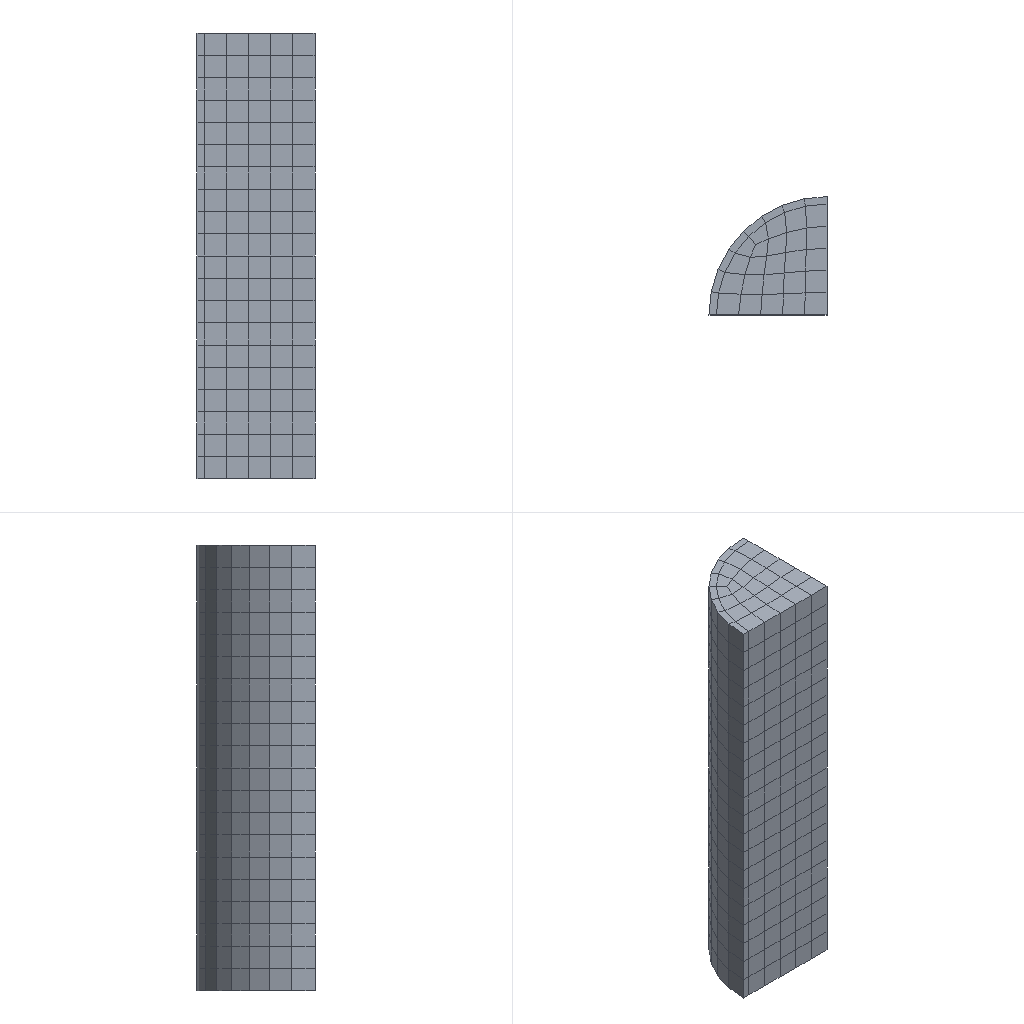Simulation study | abaqus
Set-up summary:
category,name,step,type,value,unit,region
solver,abaqus
solver,version,,,Abaqus/Explicit 2020
units,not stated in the deck,,not stated
analysis,deck,,dynamic temperature-displacement,dynamic temperature-displacement
load_step,zhazhi,zhazhi,dynamic temperature-displacement
load_step,requested,,,1
mesh,nodes,,,7514
mesh,elements,,,6802
element_type,R3D4,,rigid,6162
element_type,C3D8T,,solid,640
load,load commands in deck,,count,9
bc,support commands in deck,,count,39
material,MNSIV_R,,in results
material,SI-20MNSIV-1200-NEW,,in results
material,SUS304-1200-NEW,,in results
material,SUS304_R,,in results
check,setup vs results,,match,"per instance, exact: element labels, types and connectivity; labels of the nodes the elements use; coordinates not compared"
Abaqus input file, long lists of numbers shortened:
*Heading
** Job name: Job-1 Model name: Model-1
** Generated by: Abaqus/CAE 2020
*Preprint, echo=NO, model=NO, history=NO, contact=NO
**
** PARTS
**
*Part, name=K1
*Node
      1,         265.,  -42.456,           0.
      2,         265.,        -200.,           0.
** (1129 more lines like these left out)
*Element, type=R3D4
  1,   1,  46, 334,  47
  2,  46,  45, 335, 334
** (1090 more lines like these left out)
*Node
   1132,           0.,   8.485, -1.46030123e-14
*Nset, nset=K1-RefPt_, internal
1132,
*End Part
**
*Part, name=K2
*Node
      1,         265.,  -70.228,           0.
      2,         265.,        -200.,           0.
** (918 more lines like these left out)
*Element, type=R3D4
  1,   1,  46, 258,  47
  2,  46,  45, 259, 258
** (878 more lines like these left out)
*Node
    921,           0.,   65.418, -1.61510785e-14
*Nset, nset=K2-RefPt_, internal
921,
*End Part
**
*Part, name=K3
*Node
      1,         300.,   -56.441,           0.
      2,         300.,        -200.,           0.
** (1159 more lines like these left out)
*Element, type=R3D4
  1,   1,  50, 364,  51
  2,  50,  49, 365, 364
** (1116 more lines like these left out)
*Node
   1162,           0.,   39.471, -1.79392735e-14
*Nset, nset=K3-RefPt_, internal
1162,
*End Part
**
*Part, name=K4
*Node
      1,         300.,  -91.246,           0.
      2,         300.,        -200.,           0.
** (1033 more lines like these left out)
*Element, type=R3D4
  1,   1,  51, 288,  52
  2,  51,  50, 289, 288
** (988 more lines like these left out)
*Node
   1036,           0.,   83.469, -1.82366261e-14
*Nset, nset=K4-RefPt_, internal
1036,
*End Part
**
*Part, name=K5
*Node
      1,         300.,   -76.534,           0.
      2,         300.,        -200.,           0.
** (1132 more lines like these left out)
*Element, type=R3D4
  1,   1,  49, 356,  50
  2,  49,  48, 357, 356
** (1090 more lines like these left out)
*Node
   1135,           0.,   53.28, -1.77827639e-14
*Nset, nset=K5-RefPt_, internal
1135,
*End Part
**
*Part, name=K6
*Node
      1,         300.,  -107.209,           0.
      2,         300.,        -200.,           0.
** (1033 more lines like these left out)
*Element, type=R3D4
 1,   1,  51, 288,  52
 2,  51,  50, 289, 288
** (988 more lines like these left out)
*Node
   1036,           0.,   94.743, -1.81027001e-14
*Nset, nset=K6-RefPt_, internal
1036,
*End Part
**
*Part, name=buxiugang
*Node
      1,        -79.5,           0.,         300.
      2,  -77.972,   15.51,         300.
** (376 more lines like these left out)
*Element, type=C3D8T
  1, 190, 191, 200, 199,   1,   2,  11,  10
  2, 191, 192, 201, 200,   2,   3,  12,  11
** (158 more lines like these left out)
*Nset, nset=Set-1, generate
   1,  378,    1
*Elset, elset=Set-1, generate
   1,  160,    1
*Nset, nset=Set-3, generate
   1,  378,    1
*Elset, elset=Set-3, generate
   1,  160,    1
** Section: buxiugang
*Solid Section, elset=Set-3, material=SUS304_R
,
*End Part
**
*Part, name=tangang
*Node
      1,           0.,         74.5,         150.
      2,           0.,         74.5,         300.
** (712 more lines like these left out)
*Element, type=C3D8T
  1,  61, 202, 229,  60,   1,  22,  39,   4
  2, 202, 203, 230, 229,  22,  23,  38,  39
** (478 more lines like these left out)
*Nset, nset=Set-1, generate
   1,  714,    1
*Elset, elset=Set-1, generate
   1,  480,    1
*Nset, nset=Set-4, generate
   1,  714,    1
*Elset, elset=Set-4, generate
   1,  480,    1
** Section: tangang
*Solid Section, elset=Set-4, material=mnsiv_R
,
*End Part
**
**
** ASSEMBLY
**
*Assembly, name=Assembly
**
*Instance, name=buxiugang-1, part=buxiugang
*End Instance
**
*Instance, name=tangang-1, part=tangang
*End Instance
**
*Instance, name=K6-1, part=K6
      -312.5, 1.8982025386784e-14,        -250.
      -312.5, 1.8982025386784e-14,        -250.,       -312.5, 1.8982025386784e-14,        -249.,         180.
*End Instance
**
*Instance, name=K5-1, part=K5
          0.,         310.,        -900.
          0.,         310.,        -900.,           0.,         310., -899., 90.
*End Instance
**
*Instance, name=K4-1, part=K4
      -308.5,           0.,       -1650.
*End Instance
**
*Instance, name=K3-1, part=K3
          0.,        307.5,       -2400.
          0.,        307.5,       -2400.,           0.,        307.5, -2399., 90.
*End Instance
**
*Instance, name=K2-1, part=K2
       -271.,           0.,       -3200.
*End Instance
**
*Instance, name=K1-1, part=K1
          0.,         275.,       -4000.
          0.,         275.,       -4000.,           0.,         275., -3999., 90.
*End Instance
**
*Nset, nset=Set-3, instance=K6-1
 1036,
*Nset, nset=Set-4, instance=K5-1
 1135,
*Nset, nset=Set-5, instance=K6-1
 1036,
*Nset, nset=Set-5, instance=K5-1
 1135,
*Nset, nset=Set-6, instance=buxiugang-1, generate
   9,  378,    9
*Nset, nset=Set-6, instance=tangang-1
   1,   2,   3,   4,   9,  10,  13,  14,  17,  22,  23,  24,  25,  26,  27,  28
  29,  30,  31,  32,  33,  34,  35,  36,  37,  38,  39,  70,  71,  72,  73,  74
** (6 more lines like these left out)
*Elset, elset=Set-6, instance=buxiugang-1, generate
   8,  160,    8
*Elset, elset=Set-6, instance=tangang-1
   1,   2,   3,   4,   5,   6,   7,   8,   9,  10,  41,  42,  43,  44,  45,  46
  47,  48,  49,  50,  51,  52,  53,  54,  55,  56,  57,  58,  59,  60,  61,  62
** (5 more lines like these left out)
*Nset, nset=Set-7, instance=buxiugang-1, generate
   1,  370,    9
*Nset, nset=Set-7, instance=tangang-1
   9,  10,  11,  12,  13,  15,  19,  20,  21,  73,  74,  75,  76,  77,  78,  79
  80,  81,  88,  89,  90,  91,  92,  93,  94,  95,  96, 100, 101, 102, 103, 104
** (6 more lines like these left out)
*Elset, elset=Set-7, instance=buxiugang-1, generate
   1,  153,    8
*Elset, elset=Set-7, instance=tangang-1
  44,  48,  52,  56,  60,  64,  68,  72,  76,  80,  84,  88,  92,  96, 100, 104
 108, 112, 116, 120, 124, 128, 132, 136, 140, 144, 148, 152, 156, 160, 164, 168
** (5 more lines like these left out)
*Nset, nset=Set-8, instance=buxiugang-1, generate
   1,  378,    1
*Nset, nset=Set-8, instance=tangang-1, generate
   1,  714,    1
*Elset, elset=Set-8, instance=buxiugang-1, generate
   1,  160,    1
*Elset, elset=Set-8, instance=tangang-1, generate
   1,  480,    1
*Nset, nset=Set-9, instance=buxiugang-1, generate
   1,  378,    1
*Nset, nset=Set-9, instance=tangang-1, generate
   1,  714,    1
*Elset, elset=Set-9, instance=buxiugang-1, generate
   1,  160,    1
*Elset, elset=Set-9, instance=tangang-1, generate
   1,  480,    1
*Nset, nset=Set-10, instance=K6-1
 1036,
*Nset, nset=Set-10, instance=K5-1
 1135,
*Nset, nset=Set-10, instance=K3-1
 1162,
*Nset, nset=Set-10, instance=K1-1
 1132,
*Nset, nset=Set-10, instance=K4-1
 1036,
*Nset, nset=Set-10, instance=K2-1
 921,
*Nset, nset=Set-21, instance=K4-1
 1036,
*Nset, nset=Set-22, instance=K2-1
 921,
*Nset, nset=Set-23, instance=K3-1
 1162,
*Nset, nset=Set-24, instance=K1-1
 1132,
*Nset, nset=b_Set-10, instance=K6-1, generate
    1,  1035,     1
*Elset, elset=b_Set-10, instance=K6-1, generate
   1,  990,    1
*Nset, nset=b_Set-11, instance=K5-1, generate
    1,  1134,     1
*Elset, elset=b_Set-11, instance=K5-1, generate
    1,  1092,     1
*Nset, nset=b_Set-13, instance=K4-1, generate
    1,  1035,     1
*Elset, elset=b_Set-13, instance=K4-1, generate
   1,  990,    1
*Nset, nset=b_Set-15, instance=K3-1, generate
    1,  1161,     1
*Elset, elset=b_Set-15, instance=K3-1, generate
    1,  1118,     1
*Nset, nset=b_Set-17, instance=K2-1, generate
   1,  920,    1
*Elset, elset=b_Set-17, instance=K2-1, generate
   1,  880,    1
*Nset, nset=b_Set-19, instance=K1-1, generate
    1,  1131,     1
*Elset, elset=b_Set-19, instance=K1-1, generate
    1,  1092,     1
*Nset, nset=_PickedSet37, internal, instance=K6-1
 1036,
*Nset, nset=_PickedSet39, internal, instance=K5-1
 1135,
*Nset, nset=_PickedSet60, internal, instance=K4-1
 1036,
*Nset, nset=_PickedSet62, internal, instance=K3-1
 1162,
*Nset, nset=_PickedSet64, internal, instance=K2-1
 921,
*Nset, nset=_PickedSet66, internal, instance=K1-1
 1132,
*Elset, elset=_Surf-11_S1, internal, instance=buxiugang-1, generate
   1,  160,    1
*Elset, elset=_Surf-11_S6, internal, instance=buxiugang-1, generate
   1,  153,    8
*Elset, elset=_Surf-11_S2, internal, instance=buxiugang-1, generate
   1,  160,    1
*Elset, elset=_Surf-11_S2, internal, instance=tangang-1
   1,   2,   3,   4,   5,   6,   7,   8,   9,  10,  41,  42,  43,  44,  45,  46
  47,  48,  49,  50,  51,  52,  53,  54,  55,  56,  57,  58,  59,  60,  61,  62
** (7 more lines like these left out)
*Elset, elset=_Surf-11_S4, internal, instance=buxiugang-1, generate
   8,  160,    8
*Elset, elset=_Surf-11_S4, internal, instance=tangang-1
  10,  20,  30,  40,  44,  48,  52,  56,  60,  64,  68,  72,  76,  80,  84,  88
  92,  96, 100, 104, 108, 112, 116, 120, 124, 128, 132, 136, 140, 144, 148, 152
** (6 more lines like these left out)
*Elset, elset=_Surf-11_S3, internal, instance=buxiugang-1, generate
 1,  8,  1
*Elset, elset=_Surf-11_S3, internal, instance=tangang-1
   1,   2,   3,   4,   5,   6,   7,   8,   9,  10,  11,  12,  13,  14,  15,  16
  17,  18,  19,  20,  21,  22,  23,  24,  25,  26,  27,  28,  29,  30,  31,  32
** (7 more lines like these left out)
*Elset, elset=_Surf-11_S5, internal, instance=buxiugang-1, generate
 153,  160,    1
*Surface, type=ELEMENT, name=Surf-11
_Surf-11_S1, S1
_Surf-11_S6, S6
_Surf-11_S2, S2
_Surf-11_S4, S4
_Surf-11_S3, S3
_Surf-11_S5, S5
*Elset, elset=_Surf-12_SPOS, internal, instance=K6-1, generate
   1,  990,    1
*Surface, type=ELEMENT, name=Surf-12
_Surf-12_SPOS, SPOS
*Elset, elset=_Surf-13_SPOS, internal, instance=K5-1, generate
    1,  1092,     1
*Surface, type=ELEMENT, name=Surf-13
_Surf-13_SPOS, SPOS
*Elset, elset=_Surf-14_SPOS, internal, instance=K6-1, generate
   1,  990,    1
*Surface, type=ELEMENT, name=Surf-14
_Surf-14_SPOS, SPOS
*Elset, elset=_Surf-15_SPOS, internal, instance=K5-1, generate
    1,  1092,     1
*Surface, type=ELEMENT, name=Surf-15
_Surf-15_SPOS, SPOS
*Elset, elset=_m_Surf-1_SPOS, internal, instance=K6-1, generate
   1,  990,    1
*Surface, type=ELEMENT, name=m_Surf-1
_m_Surf-1_SPOS, SPOS
*Elset, elset=_m_Surf-3_SPOS, internal, instance=K6-1, generate
   1,  990,    1
*Surface, type=ELEMENT, name=m_Surf-3
_m_Surf-3_SPOS, SPOS
*Elset, elset=_m_Surf-5_SPOS, internal, instance=K5-1, generate
    1,  1092,     1
*Surface, type=ELEMENT, name=m_Surf-5
_m_Surf-5_SPOS, SPOS
*Elset, elset=_m_Surf-7_SPOS, internal, instance=K5-1, generate
    1,  1092,     1
*Surface, type=ELEMENT, name=m_Surf-7
_m_Surf-7_SPOS, SPOS
*Elset, elset=_m_Surf-9_S1, internal, instance=buxiugang-1, generate
   1,  160,    1
*Surface, type=ELEMENT, name=m_Surf-9
_m_Surf-9_S1, S1
*Elset, elset=_m_Surf-16_S1, internal, instance=buxiugang-1, generate
   1,  160,    1
*Surface, type=ELEMENT, name=m_Surf-16
_m_Surf-16_S1, S1
*Elset, elset=_m_Surf-18_SPOS, internal, instance=K4-1, generate
   1,  990,    1
*Surface, type=ELEMENT, name=m_Surf-18
_m_Surf-18_SPOS, SPOS
*Elset, elset=_m_Surf-20_SPOS, internal, instance=K3-1, generate
    1,  1118,     1
*Surface, type=ELEMENT, name=m_Surf-20
_m_Surf-20_SPOS, SPOS
*Elset, elset=_m_Surf-22_SPOS, internal, instance=K2-1, generate
   1,  880,    1
*Surface, type=ELEMENT, name=m_Surf-22
_m_Surf-22_SPOS, SPOS
*Elset, elset=_m_Surf-24_SPOS, internal, instance=K1-1, generate
    1,  1092,     1
*Surface, type=ELEMENT, name=m_Surf-24
_m_Surf-24_SPOS, SPOS
*Elset, elset=_s_Surf-1_S2, internal, instance=buxiugang-1, generate
   1,  160,    1
*Elset, elset=_s_Surf-1_S5, internal, instance=buxiugang-1, generate
 153,  160,    1
*Surface, type=ELEMENT, name=s_Surf-1
_s_Surf-1_S2, S2
_s_Surf-1_S5, S5
*Elset, elset=_s_Surf-3_S4, internal, instance=tangang-1, generate
 210,  360,   10
*Elset, elset=_s_Surf-3_S3, internal, instance=tangang-1
 361, 371, 381, 391, 441, 442, 443, 444
*Surface, type=ELEMENT, name=s_Surf-3
_s_Surf-3_S4, S4
_s_Surf-3_S3, S3
*Elset, elset=_s_Surf-5_S2, internal, instance=buxiugang-1, generate
   1,  160,    1
*Elset, elset=_s_Surf-5_S5, internal, instance=buxiugang-1, generate
 153,  160,    1
*Surface, type=ELEMENT, name=s_Surf-5
_s_Surf-5_S2, S2
_s_Surf-5_S5, S5
*Elset, elset=_s_Surf-7_S4, internal, instance=tangang-1, generate
 210,  360,   10
*Elset, elset=_s_Surf-7_S3, internal, instance=tangang-1
 361, 371, 381, 391, 441, 442, 443, 444
*Surface, type=ELEMENT, name=s_Surf-7
_s_Surf-7_S4, S4
_s_Surf-7_S3, S3
*Elset, elset=_s_Surf-9_S3, internal, instance=tangang-1
   1,   2,   3,   4,   5,   6,   7,   8,   9,  10,  11,  12,  13,  14,  15,  16
  17,  18,  19,  20,  21,  22,  23,  24,  25,  26,  27,  28,  29,  30,  31,  32
** (3 more lines like these left out)
*Elset, elset=_s_Surf-9_S4, internal, instance=tangang-1, generate
 361,  400,    1
*Elset, elset=_s_Surf-9_S2, internal, instance=tangang-1, generate
 441,  480,    1
*Surface, type=ELEMENT, name=s_Surf-9
_s_Surf-9_S3, S3
_s_Surf-9_S4, S4
_s_Surf-9_S2, S2
*Elset, elset=_s_Surf-16_S3, internal, instance=tangang-1
   1,   2,   3,   4,   5,   6,   7,   8,   9,  10,  11,  12,  13,  14,  15,  16
  17,  18,  19,  20,  21,  22,  23,  24,  25,  26,  27,  28,  29,  30,  31,  32
** (3 more lines like these left out)
*Elset, elset=_s_Surf-16_S4, internal, instance=tangang-1, generate
 361,  400,    1
*Elset, elset=_s_Surf-16_S2, internal, instance=tangang-1, generate
 441,  480,    1
*Surface, type=ELEMENT, name=s_Surf-16
_s_Surf-16_S3, S3
_s_Surf-16_S4, S4
_s_Surf-16_S2, S2
*Elset, elset=_s_Surf-18_S2, internal, instance=buxiugang-1, generate
   1,  160,    1
*Elset, elset=_s_Surf-18_S5, internal, instance=buxiugang-1, generate
 153,  160,    1
*Surface, type=ELEMENT, name=s_Surf-18
_s_Surf-18_S2, S2
_s_Surf-18_S5, S5
*Elset, elset=_s_Surf-20_S2, internal, instance=buxiugang-1, generate
   1,  160,    1
*Elset, elset=_s_Surf-20_S5, internal, instance=buxiugang-1, generate
 153,  160,    1
*Surface, type=ELEMENT, name=s_Surf-20
_s_Surf-20_S2, S2
_s_Surf-20_S5, S5
*Elset, elset=_s_Surf-22_S2, internal, instance=buxiugang-1, generate
   1,  160,    1
*Elset, elset=_s_Surf-22_S5, internal, instance=buxiugang-1, generate
 153,  160,    1
*Surface, type=ELEMENT, name=s_Surf-22
_s_Surf-22_S2, S2
_s_Surf-22_S5, S5
*Elset, elset=_s_Surf-24_S2, internal, instance=buxiugang-1, generate
   1,  160,    1
*Elset, elset=_s_Surf-24_S5, internal, instance=buxiugang-1, generate
 153,  160,    1
*Surface, type=ELEMENT, name=s_Surf-24
_s_Surf-24_S2, S2
_s_Surf-24_S5, S5
** Constraint: Constraint-1
*Rigid Body, ref node=_PickedSet37, elset=b_Set-10, isothermal=YES
** Constraint: Constraint-2
*Rigid Body, ref node=_PickedSet39, elset=b_Set-11, isothermal=YES
** Constraint: Constraint-3
*Tie, name=Constraint-3, adjust=yes
s_Surf-16, m_Surf-16
** Constraint: Constraint-4
*Rigid Body, ref node=_PickedSet60, elset=b_Set-13, isothermal=YES
** Constraint: Constraint-5
*Rigid Body, ref node=_PickedSet62, elset=b_Set-15, isothermal=YES
** Constraint: Constraint-6
*Rigid Body, ref node=_PickedSet64, elset=b_Set-17, isothermal=YES
** Constraint: Constraint-7
*Rigid Body, ref node=_PickedSet66, elset=b_Set-19, isothermal=YES
*End Assembly
**
** MATERIALS
**
*Material, name=SUS304-1200-new
*Density
 7.93e-09,
*Elastic
202000., 0.3
*Plastic
   27.,    0.
  55.6, 0.008
  66.7, 0.012
  71.4, 0.018
   75., 0.025
  83.3,  0.04
  90.2,  0.05
  98.5, 0.075
 104.2,   0.1
 112.5,  0.15
 116.7,   0.2
 118.8,  0.25
  114.,   0.3
 113.9,  0.35
 108.3,   0.4
 105.6,  0.45
 102.2,   0.5
   95.,  0.55
  92.2,   0.6
  85.3,  0.65
  81.9,   0.7
*Material, name=SUS304_R
*Conductivity
 600., 22.652
 650., 23.288
 700., 23.924
 750., 24.56
 800., 25.196
 850., 25.832
 900., 26.468
 950., 27.104
1000., 27.739
1050., 28.375
1100., 29.011
1150., 29.647
1200., 30.283
*Density
 7.93e-09,
*Elastic
 149257.,  0.3, 600.
 145298.,  0.3, 650.
 141301.,  0.3, 700.
 137267.,  0.3, 750.
 133197.,  0.3, 800.
 129093.,  0.3, 850.
 124956.,  0.3, 900.
 120788.,  0.3, 950.
 116590.,  0.3,1000.
 112364.,  0.3,1050.
 108111.,  0.3,1100.
 103834.,  0.3,1150.
 99534.3,  0.3,1200.
*Expansion
 2.06417e-05, 600.
 2.07678e-05, 650.
 2.08962e-05, 700.
 2.10269e-05, 750.
 2.11599e-05, 800.
 2.12952e-05, 850.
 2.14329e-05, 900.
 2.15728e-05, 950.
  2.1715e-05,1000.
 2.18595e-05,1050.
 2.20064e-05,1100.
 2.21555e-05,1150.
 2.23069e-05,1200.
*Inelastic Heat Fraction
         0.9,
*Plastic
 229.978,   0., 600.
 316.183, 0.02, 600.
 347.981, 0.04, 600.
 368.045, 0.06, 600.
 382.978, 0.08, 600.
 394.977,  0.1, 600.
  405.06, 0.12, 600.
 413.785, 0.14, 600.
 421.495, 0.16, 600.
 428.414, 0.18, 600.
   434.7,  0.2, 600.
 440.466, 0.22, 600.
 445.797, 0.24, 600.
 450.757, 0.26, 600.
 455.399, 0.28, 600.
 459.764,  0.3, 600.
 463.885, 0.32, 600.
 467.789, 0.34, 600.
   471.5, 0.36, 600.
 475.038, 0.38, 600.
 478.419,  0.4, 600.
 481.657, 0.42, 600.
 484.764, 0.44, 600.
 487.753, 0.46, 600.
 490.631, 0.48, 600.
 493.408,  0.5, 600.
 506.003,  0.6, 600.
 516.902,  0.7, 600.
 526.534,  0.8, 600.
 535.178,  0.9, 600.
  543.03,   1., 600.
 163.664,   0., 800.
 261.302, 0.02, 800.
 299.027, 0.04, 800.
  323.87, 0.06, 800.
 342.827, 0.08, 800.
 358.332,  0.1, 800.
  371.54, 0.12, 800.
 383.099, 0.14, 800.
 393.411, 0.16, 800.
** (146 more lines like these left out)
*Specific Heat
 5.8302e+08, 600.
 5.8594e+08, 650.
 5.9186e+08, 700.
  5.992e+08, 750.
 6.0726e+08, 800.
  6.158e+08, 850.
 6.2472e+08, 900.
  6.339e+08, 950.
 6.4336e+08,1000.
 6.5304e+08,1050.
 6.6296e+08,1100.
 6.7304e+08,1150.
*Material, name=Si-20MnSiV-1200-new
*Density
 7.4e-09,
*Elastic
210000., 0.3
*Plastic
 6.23,    0.
 27.1, 0.025
 38.9,  0.05
 57.6, 0.075
 70.8,   0.1
 82.6, 0.125
 88.2,  0.15
 89.5, 0.175
 90.9,   0.2
 91.6,  0.25
 92.3,   0.3
 91.6,  0.35
 89.5,   0.4
 85.5,  0.45
  82.,   0.5
*Material, name=mnsiv_R
*Conductivity
 34.288,   600.
 33.05,   650.
 32.109, 693.81
 31.484,   700.
 30.258,   709.
 28.888,   750.
 27.258, 797.31
 27.167,   800.
 26.711, 813.67
 27.148,   850.
 27.75,   900.
 28.352,   950.
 28.954,  1000.
 29.555,  1050.
 30.156,  1100.
 30.757,  1150.
 31.358,  1200.
*Density
 7.4e-09,
*Elastic
 157489.,    0.3,   600.
 150379.,    0.3,   650.
 143951.,    0.3, 693.81
 142278.,    0.3,   700.
 139622.,    0.3,   709.
 133332.,    0.3,   750.
 126645.,    0.3, 797.31
 126296.,    0.3,   800.
 124523.,    0.3, 813.67
 120961.,    0.3,   850.
 116030.,    0.3,   900.
 111066.,    0.3,   950.
 106069.,    0.3,  1000.
 101040.,    0.3,  1050.
 95977.7,    0.3,  1100.
 90882.8,    0.3,  1150.
 85755.2,    0.3,  1200.
*Expansion
 1.46737e-05,   600.
 1.49145e-05,   650.
  1.5126e-05, 693.81
 1.48211e-05,   700.
 1.41673e-05,   709.
 1.33824e-05,   750.
 1.18574e-05, 797.31
 1.17471e-05,   800.
 1.11595e-05, 813.67
 1.17592e-05,   850.
 1.25054e-05,   900.
 1.31737e-05,   950.
 1.37761e-05,  1000.
 1.43226e-05,  1050.
 1.48212e-05,  1100.
 1.52787e-05,  1150.
 1.57008e-05,  1200.
*Inelastic Heat Fraction
         0.9,
*Plastic
 270.765,   0., 600.
 376.822, 0.02, 600.
 415.606, 0.04, 600.
 440.223, 0.06, 600.
 458.599, 0.08, 600.
 473.392,  0.1, 600.
  485.84, 0.12, 600.
 496.623, 0.14, 600.
 506.161, 0.16, 600.
 514.727, 0.18, 600.
 522.514,  0.2, 600.
  529.66, 0.22, 600.
  536.27, 0.24, 600.
 542.424, 0.26, 600.
 548.186, 0.28, 600.
 553.605,  0.3, 600.
 558.722, 0.32, 600.
 563.573, 0.34, 600.
 568.186, 0.36, 600.
 572.584, 0.38, 600.
 576.787,  0.4, 600.
 580.815, 0.42, 600.
 584.681, 0.44, 600.
   588.4, 0.46, 600.
 591.982, 0.48, 600.
 595.439,  0.5, 600.
 611.128,  0.6, 600.
 120.189,   0., 800.
 191.636, 0.02, 800.
 191.636, 0.04, 800.
 191.634, 0.06, 800.
 191.627, 0.08, 800.
 191.618,  0.1, 800.
 191.597, 0.12, 800.
 191.565, 0.14, 800.
 191.516, 0.16, 800.
 191.447, 0.18, 800.
 191.354,  0.2, 800.
 191.236, 0.22, 800.
 191.091, 0.24, 800.
** (122 more lines like these left out)
*Specific Heat
  8.0543e+08, 600.
  8.7596e+08, 650.
 2.19984e+09, 700.
 1.10745e+09, 750.
  9.7917e+08, 800.
  6.0335e+08, 850.
  6.1105e+08, 900.
  6.1881e+08, 950.
  6.2658e+08,1000.
  6.3439e+08,1050.
  6.4224e+08,1100.
  6.5018e+08,1150.
  6.5806e+08,1200.
**
** INTERACTION PROPERTIES
**
*Surface Interaction, name=IntProp-1
*Friction
 0.2,
*Gap Conductance
15., 0.
 0.,10.
**
** PREDEFINED FIELDS
**
** Name: Predefined Field-1   Type: Temperature
*Initial Conditions, type=TEMPERATURE
Set-8, 1200.
** Name: Predefined Field-2   Type: Velocity
*Initial Conditions, type=VELOCITY
Set-9, 1, 0.
Set-9, 2, 0.
Set-9, 3, -600.
** ----------------------------------------------------------------
**
** STEP: zhazhi
**
*Step, name=zhazhi, nlgeom=YES
*Dynamic Temperature-displacement, Explicit
, 12.
*Bulk Viscosity
0.06, 1.2
** Mass Scaling: Semi-Automatic
**               Whole Model
*Fixed Mass Scaling, factor=10000.
**
** BOUNDARY CONDITIONS
**
** Name: BC-1 Type: 速度/角速度
*Boundary, type=VELOCITY
Set-3, 1, 1
Set-3, 2, 2
Set-3, 3, 3
Set-3, 4, 4
Set-3, 5, 5, 2.
Set-3, 6, 6
** Name: BC-2 Type: 速度/角速度
*Boundary, type=VELOCITY
Set-4, 1, 1
Set-4, 2, 2
Set-4, 3, 3
Set-4, 4, 4, 2.
Set-4, 5, 5
Set-4, 6, 6
** Name: BC-3 Type: 温度
*Boundary
Set-10, 11, 11, 200.
** Name: BC-4 Type: 位移/转角
*Boundary
Set-6, 1, 1
** Name: BC-5 Type: 对称/反对称/完全固定
*Boundary
Set-7, YSYMM
** Name: BC-6 Type: 速度/角速度
*Boundary, type=VELOCITY
Set-21, 1, 1
Set-21, 2, 2
Set-21, 3, 3
Set-21, 4, 4
Set-21, 5, 5, 2.
Set-21, 6, 6
** Name: BC-7 Type: 速度/角速度
*Boundary, type=VELOCITY
Set-22, 1, 1
Set-22, 2, 2
Set-22, 3, 3
Set-22, 4, 4
Set-22, 5, 5, 2.264
Set-22, 6, 6
** Name: BC-8 Type: 速度/角速度
*Boundary, type=VELOCITY
Set-23, 1, 1
Set-23, 2, 2
Set-23, 3, 3
Set-23, 4, 4, 2.
Set-23, 5, 5
Set-23, 6, 6
** Name: BC-9 Type: 速度/角速度
*Boundary, type=VELOCITY
Set-24, 1, 1
Set-24, 2, 2
Set-24, 3, 3
Set-24, 4, 4, 2.264
Set-24, 5, 5
Set-24, 6, 6
**
** INTERACTIONS
**
** Interaction: Int-1
*Contact Pair, interaction=IntProp-1, mechanical constraint=KINEMATIC, cpset=Int-1
m_Surf-1, s_Surf-1
** Interaction: Int-3
*Contact Pair, interaction=IntProp-1, mechanical constraint=KINEMATIC, cpset=Int-3
m_Surf-5, s_Surf-5
** Interaction: Int-4
*Contact Pair, interaction=IntProp-1, mechanical constraint=KINEMATIC, cpset=Int-4
m_Surf-18, s_Surf-18
** Interaction: Int-5
*Contact Pair, interaction=IntProp-1, mechanical constraint=KINEMATIC, cpset=Int-5
m_Surf-20, s_Surf-20
** Interaction: Int-7
*Contact Pair, interaction=IntProp-1, mechanical constraint=KINEMATIC, cpset=Int-7
m_Surf-22, s_Surf-22
** Interaction: Int-8
*Contact Pair, interaction=IntProp-1, mechanical constraint=KINEMATIC, cpset=Int-8
m_Surf-24, s_Surf-24
** Interaction: Int-6
*Sfilm
Surf-11, F, 20., 0.17
**
** OUTPUT REQUESTS
**
*Restart, write, number interval=1, time marks=NO
**
** FIELD OUTPUT: F-Output-1
**
*Output, field, variable=PRESELECT
**
** HISTORY OUTPUT: H-Output-1
**
*Output, history, variable=PRESELECT
*End Step
Results summary:
result,step,zhazhi,completed,increments=296217 time=12.0/12.0
result,analysis,,,"dynamic temperature-displacement, explict"
result,last_loadstep,,,1
result,primary field,,,"U, NT11"
result,reaction total,,FX,-437578.507,model units
result,reaction total,,FY,207245.474,model units
result,reaction total,,FZ,0.0,model units